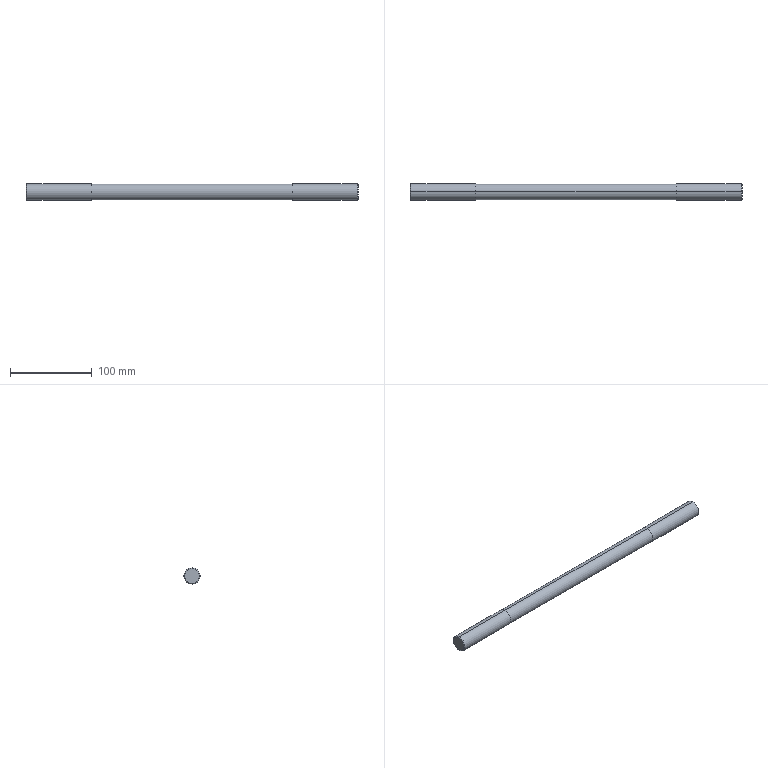Part | SolidWorks | features Chamfer 1, Revolution 1 | 1 solid | 14 faces | box 405 x 20 x 20 mm | volume 123373 mm3 | cylinder 6 | cone 4 | plane 4 | commonest cylinder face diameters 20 x4 19.5 x2
STEP:
#1=CARTESIAN_POINT('',(0.,0.,9.));
#2=VERTEX_POINT('',#1);
#3=CARTESIAN_POINT('',(0.,0.,-9.));
#4=VERTEX_POINT('',#3);
#5=CARTESIAN_POINT('',(0.,0.,0.));
#6=DIRECTION('',(-1.,0.,0.));
#7=DIRECTION('',(0.,0.,-1.));
#8=AXIS2_PLACEMENT_3D('',#5,#6,#7);
#9=CIRCLE('',#8,9.);
#10=EDGE_CURVE('',#2,#4,#9,.T.);
#11=ORIENTED_EDGE('',*,*,#10,.F.);
#12=CARTESIAN_POINT('',(1.,0.,10.));
#13=VERTEX_POINT('',#12);
#14=CARTESIAN_POINT('',(0.,0.,9.));
#15=DIRECTION('',(0.7071,0.,0.7071));
#16=VECTOR('',#15,1000.);
#17=LINE('',#14,#16);
#18=EDGE_CURVE('',#2,#13,#17,.T.);
#19=ORIENTED_EDGE('',*,*,#18,.T.);
#20=CARTESIAN_POINT('',(1.,0.,-10.));
#21=VERTEX_POINT('',#20);
#22=CARTESIAN_POINT('',(1.,0.,0.));
#23=DIRECTION('',(1.,0.,0.));
#24=DIRECTION('',(0.,0.,-1.));
#25=AXIS2_PLACEMENT_3D('',#22,#23,#24);
#26=CIRCLE('',#25,10.);
#27=EDGE_CURVE('',#21,#13,#26,.T.);
#28=ORIENTED_EDGE('',*,*,#27,.F.);
#29=CARTESIAN_POINT('',(0.,0.,-9.));
#30=DIRECTION('',(0.7071,0.,-0.7071));
#31=VECTOR('',#30,1000.);
#32=LINE('',#29,#31);
#33=EDGE_CURVE('',#4,#21,#32,.T.);
#34=ORIENTED_EDGE('',*,*,#33,.F.);
#35=EDGE_LOOP('',(#11,#19,#28,#34));
#36=FACE_OUTER_BOUND('',#35,.T.);
#37=CARTESIAN_POINT('',(0.,0.,0.));
#38=DIRECTION('',(1.,0.,0.));
#39=DIRECTION('',(0.,0.,-1.));
#40=AXIS2_PLACEMENT_3D('',#37,#38,#39);
#41=CONICAL_SURFACE('',#40,9.,0.7854);
#42=ADVANCED_FACE('',(#36),#41,.T.);
#43=CARTESIAN_POINT('',(405.,0.,-9.));
#44=VERTEX_POINT('',#43);
#45=CARTESIAN_POINT('',(405.,0.,9.));
#46=VERTEX_POINT('',#45);
#47=CARTESIAN_POINT('',(405.,0.,0.));
#48=DIRECTION('',(1.,0.,0.));
#49=DIRECTION('',(0.,0.,1.));
#50=AXIS2_PLACEMENT_3D('',#47,#48,#49);
#51=CIRCLE('',#50,9.);
#52=EDGE_CURVE('',#44,#46,#51,.T.);
#53=ORIENTED_EDGE('',*,*,#52,.F.);
#54=CARTESIAN_POINT('',(404.,0.,-10.));
#55=VERTEX_POINT('',#54);
#56=CARTESIAN_POINT('',(404.,0.,-10.));
#57=DIRECTION('',(-0.7071,0.,-0.7071));
#58=VECTOR('',#57,1000.);
#59=LINE('',#56,#58);
#60=EDGE_CURVE('',#44,#55,#59,.T.);
#61=ORIENTED_EDGE('',*,*,#60,.T.);
#62=CARTESIAN_POINT('',(404.,0.,10.));
#63=VERTEX_POINT('',#62);
#64=CARTESIAN_POINT('',(404.,0.,0.));
#65=DIRECTION('',(-1.,0.,0.));
#66=DIRECTION('',(0.,0.,1.));
#67=AXIS2_PLACEMENT_3D('',#64,#65,#66);
#68=CIRCLE('',#67,10.);
#69=EDGE_CURVE('',#63,#55,#68,.T.);
#70=ORIENTED_EDGE('',*,*,#69,.F.);
#71=CARTESIAN_POINT('',(404.,0.,10.));
#72=DIRECTION('',(-0.7071,0.,0.7071));
#73=VECTOR('',#72,1000.);
#74=LINE('',#71,#73);
#75=EDGE_CURVE('',#46,#63,#74,.T.);
#76=ORIENTED_EDGE('',*,*,#75,.F.);
#77=EDGE_LOOP('',(#53,#61,#70,#76));
#78=FACE_OUTER_BOUND('',#77,.T.);
#79=CARTESIAN_POINT('',(404.,0.,0.));
#80=DIRECTION('',(-1.,0.,0.));
#81=DIRECTION('',(0.,0.,1.));
#82=AXIS2_PLACEMENT_3D('',#79,#80,#81);
#83=CONICAL_SURFACE('',#82,10.,0.7854);
#84=ADVANCED_FACE('',(#78),#83,.T.);
#85=ORIENTED_EDGE('',*,*,#69,.T.);
#86=CARTESIAN_POINT('',(325.,0.,-10.));
#87=VERTEX_POINT('',#86);
#88=CARTESIAN_POINT('',(0.,0.,-10.));
#89=DIRECTION('',(-1.,0.,0.));
#90=VECTOR('',#89,1000.);
#91=LINE('',#88,#90);
#92=EDGE_CURVE('',#55,#87,#91,.T.);
#93=ORIENTED_EDGE('',*,*,#92,.T.);
#94=CARTESIAN_POINT('',(325.,0.,10.));
#95=VERTEX_POINT('',#94);
#96=CARTESIAN_POINT('',(325.,0.,0.));
#97=DIRECTION('',(-1.,0.,0.));
#98=DIRECTION('',(0.,0.,1.));
#99=AXIS2_PLACEMENT_3D('',#96,#97,#98);
#100=CIRCLE('',#99,10.);
#101=EDGE_CURVE('',#95,#87,#100,.T.);
#102=ORIENTED_EDGE('',*,*,#101,.F.);
#103=CARTESIAN_POINT('',(0.,0.,10.));
#104=DIRECTION('',(-1.,0.,0.));
#105=VECTOR('',#104,1000.);
#106=LINE('',#103,#105);
#107=EDGE_CURVE('',#63,#95,#106,.T.);
#108=ORIENTED_EDGE('',*,*,#107,.F.);
#109=EDGE_LOOP('',(#85,#93,#102,#108));
#110=FACE_OUTER_BOUND('',#109,.T.);
#111=CARTESIAN_POINT('',(0.,0.,0.));
#112=DIRECTION('',(-1.,0.,0.));
#113=DIRECTION('',(0.,0.,1.));
#114=AXIS2_PLACEMENT_3D('',#111,#112,#113);
#115=CYLINDRICAL_SURFACE('',#114,10.);
#116=ADVANCED_FACE('',(#110),#115,.T.);
#117=CARTESIAN_POINT('',(325.,0.,9.75));
#118=VERTEX_POINT('',#117);
#119=CARTESIAN_POINT('',(325.,0.,-9.75));
#120=VERTEX_POINT('',#119);
#121=CARTESIAN_POINT('',(325.,0.,0.));
#122=DIRECTION('',(-1.,0.,0.));
#123=DIRECTION('',(0.,0.,1.));
#124=AXIS2_PLACEMENT_3D('',#121,#122,#123);
#125=CIRCLE('',#124,9.75);
#126=EDGE_CURVE('',#118,#120,#125,.T.);
#127=ORIENTED_EDGE('',*,*,#126,.T.);
#128=CARTESIAN_POINT('',(80.,0.,-9.75));
#129=VERTEX_POINT('',#128);
#130=CARTESIAN_POINT('',(0.,0.,-9.75));
#131=DIRECTION('',(-1.,0.,0.));
#132=VECTOR('',#131,1000.);
#133=LINE('',#130,#132);
#134=EDGE_CURVE('',#120,#129,#133,.T.);
#135=ORIENTED_EDGE('',*,*,#134,.T.);
#136=CARTESIAN_POINT('',(80.,0.,9.75));
#137=VERTEX_POINT('',#136);
#138=CARTESIAN_POINT('',(80.,0.,0.));
#139=DIRECTION('',(-1.,0.,0.));
#140=DIRECTION('',(0.,0.,1.));
#141=AXIS2_PLACEMENT_3D('',#138,#139,#140);
#142=CIRCLE('',#141,9.75);
#143=EDGE_CURVE('',#137,#129,#142,.T.);
#144=ORIENTED_EDGE('',*,*,#143,.F.);
#145=CARTESIAN_POINT('',(0.,0.,9.75));
#146=DIRECTION('',(-1.,0.,0.));
#147=VECTOR('',#146,1000.);
#148=LINE('',#145,#147);
#149=EDGE_CURVE('',#118,#137,#148,.T.);
#150=ORIENTED_EDGE('',*,*,#149,.F.);
#151=EDGE_LOOP('',(#127,#135,#144,#150));
#152=FACE_OUTER_BOUND('',#151,.T.);
#153=CARTESIAN_POINT('',(0.,0.,0.));
#154=DIRECTION('',(-1.,0.,0.));
#155=DIRECTION('',(0.,0.,1.));
#156=AXIS2_PLACEMENT_3D('',#153,#154,#155);
#157=CYLINDRICAL_SURFACE('',#156,9.75);
#158=ADVANCED_FACE('',(#152),#157,.T.);
#159=CARTESIAN_POINT('',(80.,0.,10.));
#160=VERTEX_POINT('',#159);
#161=CARTESIAN_POINT('',(80.,0.,-10.));
#162=VERTEX_POINT('',#161);
#163=CARTESIAN_POINT('',(80.,0.,0.));
#164=DIRECTION('',(-1.,0.,0.));
#165=DIRECTION('',(0.,0.,1.));
#166=AXIS2_PLACEMENT_3D('',#163,#164,#165);
#167=CIRCLE('',#166,10.);
#168=EDGE_CURVE('',#160,#162,#167,.T.);
#169=ORIENTED_EDGE('',*,*,#168,.T.);
#170=CARTESIAN_POINT('',(0.,0.,-10.));
#171=DIRECTION('',(-1.,0.,0.));
#172=VECTOR('',#171,1000.);
#173=LINE('',#170,#172);
#174=EDGE_CURVE('',#162,#21,#173,.T.);
#175=ORIENTED_EDGE('',*,*,#174,.T.);
#176=ORIENTED_EDGE('',*,*,#27,.T.);
#177=CARTESIAN_POINT('',(0.,0.,10.));
#178=DIRECTION('',(-1.,0.,0.));
#179=VECTOR('',#178,1000.);
#180=LINE('',#177,#179);
#181=EDGE_CURVE('',#160,#13,#180,.T.);
#182=ORIENTED_EDGE('',*,*,#181,.F.);
#183=EDGE_LOOP('',(#169,#175,#176,#182));
#184=FACE_OUTER_BOUND('',#183,.T.);
#185=CARTESIAN_POINT('',(0.,0.,0.));
#186=DIRECTION('',(-1.,0.,0.));
#187=DIRECTION('',(0.,0.,1.));
#188=AXIS2_PLACEMENT_3D('',#185,#186,#187);
#189=CYLINDRICAL_SURFACE('',#188,10.);
#190=ADVANCED_FACE('',(#184),#189,.T.);
#191=CARTESIAN_POINT('',(0.,0.,0.));
#192=DIRECTION('',(-1.,0.,0.));
#193=DIRECTION('',(0.,0.,-1.));
#194=AXIS2_PLACEMENT_3D('',#191,#192,#193);
#195=CIRCLE('',#194,9.);
#196=EDGE_CURVE('',#4,#2,#195,.T.);
#197=ORIENTED_EDGE('',*,*,#196,.T.);
#198=ORIENTED_EDGE('',*,*,#10,.T.);
#199=EDGE_LOOP('',(#197,#198));
#200=FACE_OUTER_BOUND('',#199,.T.);
#201=CARTESIAN_POINT('',(0.,0.,0.));
#202=DIRECTION('',(1.,0.,0.));
#203=DIRECTION('',(0.,0.,-1.));
#204=AXIS2_PLACEMENT_3D('',#201,#202,#203);
#205=PLANE('',#204);
#206=ADVANCED_FACE('',(#200),#205,.F.);
#207=ORIENTED_EDGE('',*,*,#174,.F.);
#208=CARTESIAN_POINT('',(80.,0.,0.));
#209=DIRECTION('',(-1.,0.,0.));
#210=DIRECTION('',(0.,0.,1.));
#211=AXIS2_PLACEMENT_3D('',#208,#209,#210);
#212=CIRCLE('',#211,10.);
#213=EDGE_CURVE('',#162,#160,#212,.T.);
#214=ORIENTED_EDGE('',*,*,#213,.T.);
#215=ORIENTED_EDGE('',*,*,#181,.T.);
#216=CARTESIAN_POINT('',(1.,0.,0.));
#217=DIRECTION('',(1.,0.,0.));
#218=DIRECTION('',(0.,0.,-1.));
#219=AXIS2_PLACEMENT_3D('',#216,#217,#218);
#220=CIRCLE('',#219,10.);
#221=EDGE_CURVE('',#13,#21,#220,.T.);
#222=ORIENTED_EDGE('',*,*,#221,.T.);
#223=EDGE_LOOP('',(#207,#214,#215,#222));
#224=FACE_OUTER_BOUND('',#223,.T.);
#225=CARTESIAN_POINT('',(0.,0.,0.));
#226=DIRECTION('',(-1.,0.,0.));
#227=DIRECTION('',(0.,0.,1.));
#228=AXIS2_PLACEMENT_3D('',#225,#226,#227);
#229=CYLINDRICAL_SURFACE('',#228,10.);
#230=ADVANCED_FACE('',(#224),#229,.T.);
#231=ORIENTED_EDGE('',*,*,#168,.F.);
#232=ORIENTED_EDGE('',*,*,#213,.F.);
#233=EDGE_LOOP('',(#231,#232));
#234=FACE_OUTER_BOUND('',#233,.T.);
#235=ORIENTED_EDGE('',*,*,#143,.T.);
#236=CARTESIAN_POINT('',(80.,0.,0.));
#237=DIRECTION('',(-1.,0.,0.));
#238=DIRECTION('',(0.,0.,1.));
#239=AXIS2_PLACEMENT_3D('',#236,#237,#238);
#240=CIRCLE('',#239,9.75);
#241=EDGE_CURVE('',#129,#137,#240,.T.);
#242=ORIENTED_EDGE('',*,*,#241,.T.);
#243=EDGE_LOOP('',(#235,#242));
#244=FACE_BOUND('',#243,.T.);
#245=CARTESIAN_POINT('',(80.,10.,0.));
#246=DIRECTION('',(-1.,0.,0.));
#247=DIRECTION('',(0.,0.,1.));
#248=AXIS2_PLACEMENT_3D('',#245,#246,#247);
#249=PLANE('',#248);
#250=ADVANCED_FACE('',(#234,#244),#249,.F.);
#251=ORIENTED_EDGE('',*,*,#134,.F.);
#252=CARTESIAN_POINT('',(325.,0.,0.));
#253=DIRECTION('',(-1.,0.,0.));
#254=DIRECTION('',(0.,0.,1.));
#255=AXIS2_PLACEMENT_3D('',#252,#253,#254);
#256=CIRCLE('',#255,9.75);
#257=EDGE_CURVE('',#120,#118,#256,.T.);
#258=ORIENTED_EDGE('',*,*,#257,.T.);
#259=ORIENTED_EDGE('',*,*,#149,.T.);
#260=ORIENTED_EDGE('',*,*,#241,.F.);
#261=EDGE_LOOP('',(#251,#258,#259,#260));
#262=FACE_OUTER_BOUND('',#261,.T.);
#263=CARTESIAN_POINT('',(0.,0.,0.));
#264=DIRECTION('',(-1.,0.,0.));
#265=DIRECTION('',(0.,0.,1.));
#266=AXIS2_PLACEMENT_3D('',#263,#264,#265);
#267=CYLINDRICAL_SURFACE('',#266,9.75);
#268=ADVANCED_FACE('',(#262),#267,.T.);
#269=ORIENTED_EDGE('',*,*,#126,.F.);
#270=ORIENTED_EDGE('',*,*,#257,.F.);
#271=EDGE_LOOP('',(#269,#270));
#272=FACE_BOUND('',#271,.T.);
#273=ORIENTED_EDGE('',*,*,#101,.T.);
#274=CARTESIAN_POINT('',(325.,0.,0.));
#275=DIRECTION('',(-1.,0.,0.));
#276=DIRECTION('',(0.,0.,1.));
#277=AXIS2_PLACEMENT_3D('',#274,#275,#276);
#278=CIRCLE('',#277,10.);
#279=EDGE_CURVE('',#87,#95,#278,.T.);
#280=ORIENTED_EDGE('',*,*,#279,.T.);
#281=EDGE_LOOP('',(#273,#280));
#282=FACE_OUTER_BOUND('',#281,.T.);
#283=CARTESIAN_POINT('',(325.,10.,0.));
#284=DIRECTION('',(1.,0.,0.));
#285=DIRECTION('',(0.,0.,-1.));
#286=AXIS2_PLACEMENT_3D('',#283,#284,#285);
#287=PLANE('',#286);
#288=ADVANCED_FACE('',(#272,#282),#287,.F.);
#289=ORIENTED_EDGE('',*,*,#92,.F.);
#290=CARTESIAN_POINT('',(404.,0.,0.));
#291=DIRECTION('',(-1.,0.,0.));
#292=DIRECTION('',(0.,0.,1.));
#293=AXIS2_PLACEMENT_3D('',#290,#291,#292);
#294=CIRCLE('',#293,10.);
#295=EDGE_CURVE('',#55,#63,#294,.T.);
#296=ORIENTED_EDGE('',*,*,#295,.T.);
#297=ORIENTED_EDGE('',*,*,#107,.T.);
#298=ORIENTED_EDGE('',*,*,#279,.F.);
#299=EDGE_LOOP('',(#289,#296,#297,#298));
#300=FACE_OUTER_BOUND('',#299,.T.);
#301=CARTESIAN_POINT('',(0.,0.,0.));
#302=DIRECTION('',(-1.,0.,0.));
#303=DIRECTION('',(0.,0.,1.));
#304=AXIS2_PLACEMENT_3D('',#301,#302,#303);
#305=CYLINDRICAL_SURFACE('',#304,10.);
#306=ADVANCED_FACE('',(#300),#305,.T.);
#307=CARTESIAN_POINT('',(405.,0.,0.));
#308=DIRECTION('',(1.,0.,0.));
#309=DIRECTION('',(0.,0.,1.));
#310=AXIS2_PLACEMENT_3D('',#307,#308,#309);
#311=CIRCLE('',#310,9.);
#312=EDGE_CURVE('',#46,#44,#311,.T.);
#313=ORIENTED_EDGE('',*,*,#312,.T.);
#314=ORIENTED_EDGE('',*,*,#52,.T.);
#315=EDGE_LOOP('',(#313,#314));
#316=FACE_OUTER_BOUND('',#315,.T.);
#317=CARTESIAN_POINT('',(405.,0.,0.));
#318=DIRECTION('',(-1.,0.,0.));
#319=DIRECTION('',(0.,0.,1.));
#320=AXIS2_PLACEMENT_3D('',#317,#318,#319);
#321=PLANE('',#320);
#322=ADVANCED_FACE('',(#316),#321,.F.);
#323=ORIENTED_EDGE('',*,*,#60,.F.);
#324=ORIENTED_EDGE('',*,*,#312,.F.);
#325=ORIENTED_EDGE('',*,*,#75,.T.);
#326=ORIENTED_EDGE('',*,*,#295,.F.);
#327=EDGE_LOOP('',(#323,#324,#325,#326));
#328=FACE_OUTER_BOUND('',#327,.T.);
#329=CARTESIAN_POINT('',(404.,0.,0.));
#330=DIRECTION('',(-1.,0.,0.));
#331=DIRECTION('',(0.,0.,1.));
#332=AXIS2_PLACEMENT_3D('',#329,#330,#331);
#333=CONICAL_SURFACE('',#332,10.,0.7854);
#334=ADVANCED_FACE('',(#328),#333,.T.);
#335=ORIENTED_EDGE('',*,*,#18,.F.);
#336=ORIENTED_EDGE('',*,*,#196,.F.);
#337=ORIENTED_EDGE('',*,*,#33,.T.);
#338=ORIENTED_EDGE('',*,*,#221,.F.);
#339=EDGE_LOOP('',(#335,#336,#337,#338));
#340=FACE_OUTER_BOUND('',#339,.T.);
#341=CARTESIAN_POINT('',(0.,0.,0.));
#342=DIRECTION('',(1.,0.,0.));
#343=DIRECTION('',(0.,0.,-1.));
#344=AXIS2_PLACEMENT_3D('',#341,#342,#343);
#345=CONICAL_SURFACE('',#344,9.,0.7854);
#346=ADVANCED_FACE('',(#340),#345,.T.);
#347=CLOSED_SHELL('',(#42,#84,#116,#158,#190,#206,#230,#250,#268,#288,#306,#322,#334,#346));
#348=MANIFOLD_SOLID_BREP('',#347);
#349=CARTESIAN_POINT('',(0.,0.,0.));
#350=DIRECTION('',(0.,0.,1.));
#351=DIRECTION('',(1.,0.,0.));
#352=AXIS2_PLACEMENT_3D('',#349,#350,#351);
#353=(LENGTH_UNIT()NAMED_UNIT(*)SI_UNIT(.MILLI.,.METRE.));
#354=UNCERTAINTY_MEASURE_WITH_UNIT(LENGTH_MEASURE(0.00001),#353,'','');
#355=(NAMED_UNIT(*)PLANE_ANGLE_UNIT()SI_UNIT($,.RADIAN.));
#356=(NAMED_UNIT(*)SI_UNIT($,.STERADIAN.)SOLID_ANGLE_UNIT());
#357=(GEOMETRIC_REPRESENTATION_CONTEXT(3)GLOBAL_UNCERTAINTY_ASSIGNED_CONTEXT((#354))GLOBAL_UNIT_ASSIGNED_CONTEXT((#353,#355,#356))REPRESENTATION_CONTEXT('',''));
#358=ADVANCED_BREP_SHAPE_REPRESENTATION('',(#348,#352),#357);